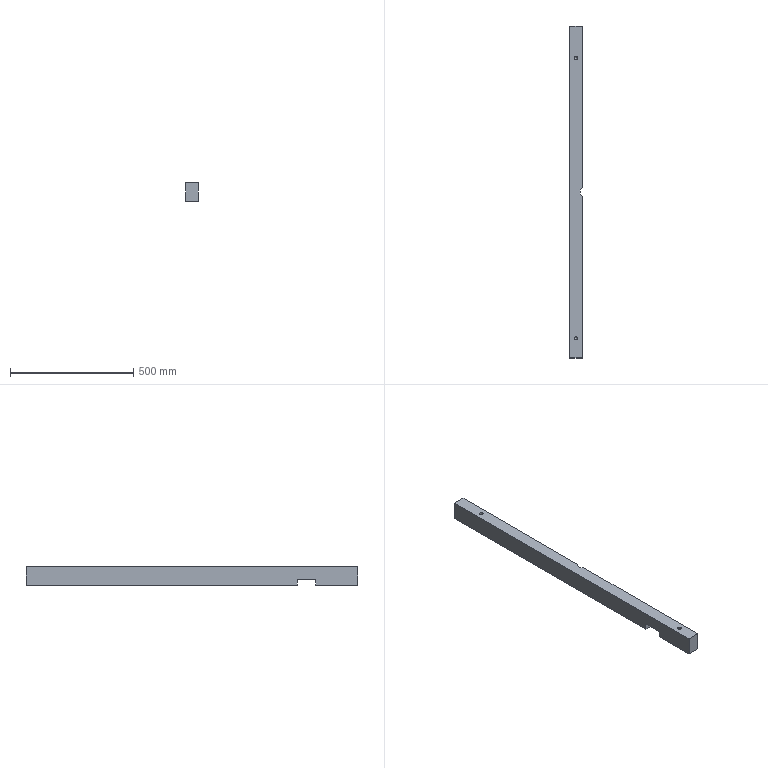Part | NX | features 3 2 | 1 solid | 20 faces | box 50 x 1345 x 75.5 mm | volume 4962481 mm3 | plane 11 | cylinder 5 | cone 4 | commonest cylinder face diameters 14.1 x4 53 x1
STEP:
#1=CARTESIAN_POINT('',(2167.05,542.5,256.5));
#2=VERTEX_POINT('',#1);
#3=CARTESIAN_POINT('',(2160.,542.5,256.5));
#4=DIRECTION('',(0.,0.,-1.));
#5=DIRECTION('',(1.,0.,0.));
#6=AXIS2_PLACEMENT_3D('',#3,#4,#5);
#7=CIRCLE('',#6,7.05);
#8=EDGE_CURVE('',#2,#2,#7,.T.);
#9=ORIENTED_EDGE('',*,*,#8,.T.);
#10=EDGE_LOOP('',(#9));
#11=FACE_BOUND('',#10,.T.);
#12=CARTESIAN_POINT('',(2185.,19.449,256.5));
#13=VERTEX_POINT('',#12);
#14=CARTESIAN_POINT('',(2185.,-19.449,256.5));
#15=VERTEX_POINT('',#14);
#16=CARTESIAN_POINT('',(2203.,0.,256.5));
#17=DIRECTION('',(0.,0.,1.));
#18=DIRECTION('',(1.,0.,0.));
#19=AXIS2_PLACEMENT_3D('',#16,#17,#18);
#20=CIRCLE('',#19,26.5);
#21=EDGE_CURVE('',#13,#15,#20,.T.);
#22=ORIENTED_EDGE('',*,*,#21,.F.);
#23=CARTESIAN_POINT('',(2185.,672.5,256.5));
#24=VERTEX_POINT('',#23);
#25=CARTESIAN_POINT('',(2185.,193.,256.5));
#26=DIRECTION('',(0.,1.,0.));
#27=VECTOR('',#26,1000.);
#28=LINE('',#25,#27);
#29=EDGE_CURVE('',#13,#24,#28,.T.);
#30=ORIENTED_EDGE('',*,*,#29,.T.);
#31=CARTESIAN_POINT('',(2135.,672.5,256.5));
#32=VERTEX_POINT('',#31);
#33=CARTESIAN_POINT('',(145.,672.5,256.5));
#34=DIRECTION('',(-1.,0.,0.));
#35=VECTOR('',#34,1000.);
#36=LINE('',#33,#35);
#37=EDGE_CURVE('',#24,#32,#36,.T.);
#38=ORIENTED_EDGE('',*,*,#37,.T.);
#39=CARTESIAN_POINT('',(2135.,-672.5,256.5));
#40=VERTEX_POINT('',#39);
#41=CARTESIAN_POINT('',(2135.,193.,256.5));
#42=DIRECTION('',(0.,-1.,0.));
#43=VECTOR('',#42,1000.);
#44=LINE('',#41,#43);
#45=EDGE_CURVE('',#32,#40,#44,.T.);
#46=ORIENTED_EDGE('',*,*,#45,.T.);
#47=CARTESIAN_POINT('',(2185.,-672.5,256.5));
#48=VERTEX_POINT('',#47);
#49=CARTESIAN_POINT('',(145.,-672.5,256.5));
#50=DIRECTION('',(1.,0.,0.));
#51=VECTOR('',#50,1000.);
#52=LINE('',#49,#51);
#53=EDGE_CURVE('',#40,#48,#52,.T.);
#54=ORIENTED_EDGE('',*,*,#53,.T.);
#55=CARTESIAN_POINT('',(2185.,193.,256.5));
#56=DIRECTION('',(0.,1.,0.));
#57=VECTOR('',#56,1000.);
#58=LINE('',#55,#57);
#59=EDGE_CURVE('',#48,#15,#58,.T.);
#60=ORIENTED_EDGE('',*,*,#59,.T.);
#61=EDGE_LOOP('',(#22,#30,#38,#46,#54,#60));
#62=FACE_BOUND('',#61,.T.);
#63=CARTESIAN_POINT('',(2167.05,-592.5,256.5));
#64=VERTEX_POINT('',#63);
#65=CARTESIAN_POINT('',(2160.,-592.5,256.5));
#66=DIRECTION('',(0.,0.,-1.));
#67=DIRECTION('',(1.,0.,0.));
#68=AXIS2_PLACEMENT_3D('',#65,#66,#67);
#69=CIRCLE('',#68,7.05);
#70=EDGE_CURVE('',#64,#64,#69,.T.);
#71=ORIENTED_EDGE('',*,*,#70,.T.);
#72=EDGE_LOOP('',(#71));
#73=FACE_BOUND('',#72,.T.);
#74=CARTESIAN_POINT('',(145.,0.,256.5));
#75=DIRECTION('',(0.,0.,1.));
#76=DIRECTION('',(1.,0.,0.));
#77=AXIS2_PLACEMENT_3D('',#74,#75,#76);
#78=PLANE('',#77);
#79=ADVANCED_FACE('',(#11,#62,#73),#78,.T.);
#80=CARTESIAN_POINT('',(2185.,-502.,181.));
#81=VERTEX_POINT('',#80);
#82=CARTESIAN_POINT('',(2135.,-502.,181.));
#83=VERTEX_POINT('',#82);
#84=CARTESIAN_POINT('',(915.,-502.,181.));
#85=DIRECTION('',(-1.,0.,0.));
#86=VECTOR('',#85,1000.);
#87=LINE('',#84,#86);
#88=EDGE_CURVE('',#81,#83,#87,.T.);
#89=ORIENTED_EDGE('',*,*,#88,.F.);
#90=CARTESIAN_POINT('',(2185.,-672.5,181.));
#91=VERTEX_POINT('',#90);
#92=CARTESIAN_POINT('',(2185.,193.,181.));
#93=DIRECTION('',(0.,-1.,0.));
#94=VECTOR('',#93,1000.);
#95=LINE('',#92,#94);
#96=EDGE_CURVE('',#81,#91,#95,.T.);
#97=ORIENTED_EDGE('',*,*,#96,.T.);
#98=CARTESIAN_POINT('',(2135.,-672.5,181.));
#99=VERTEX_POINT('',#98);
#100=CARTESIAN_POINT('',(282.5,-672.5,181.));
#101=DIRECTION('',(1.,0.,0.));
#102=VECTOR('',#101,1000.);
#103=LINE('',#100,#102);
#104=EDGE_CURVE('',#99,#91,#103,.T.);
#105=ORIENTED_EDGE('',*,*,#104,.F.);
#106=CARTESIAN_POINT('',(2135.,193.,181.));
#107=DIRECTION('',(0.,1.,0.));
#108=VECTOR('',#107,1000.);
#109=LINE('',#106,#108);
#110=EDGE_CURVE('',#99,#83,#109,.T.);
#111=ORIENTED_EDGE('',*,*,#110,.T.);
#112=EDGE_LOOP('',(#89,#97,#105,#111));
#113=FACE_BOUND('',#112,.T.);
#114=CARTESIAN_POINT('',(2167.05,-592.5,181.));
#115=VERTEX_POINT('',#114);
#116=CARTESIAN_POINT('',(2160.,-592.5,181.));
#117=DIRECTION('',(0.,0.,1.));
#118=DIRECTION('',(1.,0.,0.));
#119=AXIS2_PLACEMENT_3D('',#116,#117,#118);
#120=CIRCLE('',#119,7.05);
#121=EDGE_CURVE('',#115,#115,#120,.T.);
#122=ORIENTED_EDGE('',*,*,#121,.T.);
#123=EDGE_LOOP('',(#122));
#124=FACE_BOUND('',#123,.T.);
#125=CARTESIAN_POINT('',(915.,193.,181.));
#126=DIRECTION('',(0.,0.,-1.));
#127=DIRECTION('',(1.,0.,0.));
#128=AXIS2_PLACEMENT_3D('',#125,#126,#127);
#129=PLANE('',#128);
#130=ADVANCED_FACE('',(#113,#124),#129,.T.);
#131=CARTESIAN_POINT('',(2185.,-19.449,181.));
#132=VERTEX_POINT('',#131);
#133=CARTESIAN_POINT('',(2185.,19.449,181.));
#134=VERTEX_POINT('',#133);
#135=CARTESIAN_POINT('',(2203.,0.,181.));
#136=DIRECTION('',(0.,0.,-1.));
#137=DIRECTION('',(-1.,0.,0.));
#138=AXIS2_PLACEMENT_3D('',#135,#136,#137);
#139=CIRCLE('',#138,26.5);
#140=EDGE_CURVE('',#132,#134,#139,.T.);
#141=ORIENTED_EDGE('',*,*,#140,.F.);
#142=CARTESIAN_POINT('',(2185.,-426.,181.));
#143=VERTEX_POINT('',#142);
#144=CARTESIAN_POINT('',(2185.,193.,181.));
#145=DIRECTION('',(0.,-1.,0.));
#146=VECTOR('',#145,1000.);
#147=LINE('',#144,#146);
#148=EDGE_CURVE('',#132,#143,#147,.T.);
#149=ORIENTED_EDGE('',*,*,#148,.T.);
#150=CARTESIAN_POINT('',(2135.,-426.,181.));
#151=VERTEX_POINT('',#150);
#152=CARTESIAN_POINT('',(915.,-426.,181.));
#153=DIRECTION('',(1.,0.,0.));
#154=VECTOR('',#153,1000.);
#155=LINE('',#152,#154);
#156=EDGE_CURVE('',#151,#143,#155,.T.);
#157=ORIENTED_EDGE('',*,*,#156,.F.);
#158=CARTESIAN_POINT('',(2135.,672.5,181.));
#159=VERTEX_POINT('',#158);
#160=CARTESIAN_POINT('',(2135.,193.,181.));
#161=DIRECTION('',(0.,1.,0.));
#162=VECTOR('',#161,1000.);
#163=LINE('',#160,#162);
#164=EDGE_CURVE('',#151,#159,#163,.T.);
#165=ORIENTED_EDGE('',*,*,#164,.T.);
#166=CARTESIAN_POINT('',(2185.,672.5,181.));
#167=VERTEX_POINT('',#166);
#168=CARTESIAN_POINT('',(2185.,672.5,181.));
#169=DIRECTION('',(-1.,0.,0.));
#170=VECTOR('',#169,1000.);
#171=LINE('',#168,#170);
#172=EDGE_CURVE('',#167,#159,#171,.T.);
#173=ORIENTED_EDGE('',*,*,#172,.F.);
#174=CARTESIAN_POINT('',(2185.,193.,181.));
#175=DIRECTION('',(0.,-1.,0.));
#176=VECTOR('',#175,1000.);
#177=LINE('',#174,#176);
#178=EDGE_CURVE('',#167,#134,#177,.T.);
#179=ORIENTED_EDGE('',*,*,#178,.T.);
#180=EDGE_LOOP('',(#141,#149,#157,#165,#173,#179));
#181=FACE_BOUND('',#180,.T.);
#182=CARTESIAN_POINT('',(2167.05,542.5,181.));
#183=VERTEX_POINT('',#182);
#184=CARTESIAN_POINT('',(2160.,542.5,181.));
#185=DIRECTION('',(0.,0.,1.));
#186=DIRECTION('',(1.,0.,0.));
#187=AXIS2_PLACEMENT_3D('',#184,#185,#186);
#188=CIRCLE('',#187,7.05);
#189=EDGE_CURVE('',#183,#183,#188,.T.);
#190=ORIENTED_EDGE('',*,*,#189,.T.);
#191=EDGE_LOOP('',(#190));
#192=FACE_BOUND('',#191,.T.);
#193=CARTESIAN_POINT('',(915.,193.,181.));
#194=DIRECTION('',(0.,0.,-1.));
#195=DIRECTION('',(1.,0.,0.));
#196=AXIS2_PLACEMENT_3D('',#193,#194,#195);
#197=PLANE('',#196);
#198=ADVANCED_FACE('',(#181,#192),#197,.T.);
#199=CARTESIAN_POINT('',(2185.,19.449,-181.));
#200=DIRECTION('',(0.,0.,1.));
#201=VECTOR('',#200,1000.);
#202=LINE('',#199,#201);
#203=EDGE_CURVE('',#134,#13,#202,.T.);
#204=ORIENTED_EDGE('',*,*,#203,.F.);
#205=ORIENTED_EDGE('',*,*,#178,.F.);
#206=CARTESIAN_POINT('',(2185.,672.5,231.5));
#207=DIRECTION('',(0.,0.,-1.));
#208=VECTOR('',#207,1000.);
#209=LINE('',#206,#208);
#210=EDGE_CURVE('',#24,#167,#209,.T.);
#211=ORIENTED_EDGE('',*,*,#210,.F.);
#212=ORIENTED_EDGE('',*,*,#29,.F.);
#213=EDGE_LOOP('',(#204,#205,#211,#212));
#214=FACE_BOUND('',#213,.T.);
#215=CARTESIAN_POINT('',(2185.,193.,-1.5));
#216=DIRECTION('',(1.,0.,0.));
#217=DIRECTION('',(0.,0.,-1.));
#218=AXIS2_PLACEMENT_3D('',#215,#216,#217);
#219=PLANE('',#218);
#220=ADVANCED_FACE('',(#214),#219,.T.);
#221=CARTESIAN_POINT('',(2185.,-19.449,256.5));
#222=DIRECTION('',(0.,0.,-1.));
#223=VECTOR('',#222,1000.);
#224=LINE('',#221,#223);
#225=EDGE_CURVE('',#15,#132,#224,.T.);
#226=ORIENTED_EDGE('',*,*,#225,.F.);
#227=ORIENTED_EDGE('',*,*,#59,.F.);
#228=CARTESIAN_POINT('',(2185.,-672.5,-103.));
#229=DIRECTION('',(0.,0.,1.));
#230=VECTOR('',#229,1000.);
#231=LINE('',#228,#230);
#232=EDGE_CURVE('',#91,#48,#231,.T.);
#233=ORIENTED_EDGE('',*,*,#232,.F.);
#234=ORIENTED_EDGE('',*,*,#96,.F.);
#235=CARTESIAN_POINT('',(2185.,-502.,205.));
#236=VERTEX_POINT('',#235);
#237=CARTESIAN_POINT('',(2185.,-502.,-1.5));
#238=DIRECTION('',(0.,0.,-1.));
#239=VECTOR('',#238,1000.);
#240=LINE('',#237,#239);
#241=EDGE_CURVE('',#236,#81,#240,.T.);
#242=ORIENTED_EDGE('',*,*,#241,.F.);
#243=CARTESIAN_POINT('',(2185.,-426.,205.));
#244=VERTEX_POINT('',#243);
#245=CARTESIAN_POINT('',(2185.,193.,205.));
#246=DIRECTION('',(0.,-1.,0.));
#247=VECTOR('',#246,1000.);
#248=LINE('',#245,#247);
#249=EDGE_CURVE('',#244,#236,#248,.T.);
#250=ORIENTED_EDGE('',*,*,#249,.F.);
#251=CARTESIAN_POINT('',(2185.,-426.,-1.5));
#252=DIRECTION('',(0.,0.,1.));
#253=VECTOR('',#252,1000.);
#254=LINE('',#251,#253);
#255=EDGE_CURVE('',#143,#244,#254,.T.);
#256=ORIENTED_EDGE('',*,*,#255,.F.);
#257=ORIENTED_EDGE('',*,*,#148,.F.);
#258=EDGE_LOOP('',(#226,#227,#233,#234,#242,#250,#256,#257));
#259=FACE_BOUND('',#258,.T.);
#260=CARTESIAN_POINT('',(2185.,193.,-1.5));
#261=DIRECTION('',(1.,0.,0.));
#262=DIRECTION('',(0.,0.,-1.));
#263=AXIS2_PLACEMENT_3D('',#260,#261,#262);
#264=PLANE('',#263);
#265=ADVANCED_FACE('',(#259),#264,.T.);
#266=CARTESIAN_POINT('',(2135.,-502.,205.));
#267=VERTEX_POINT('',#266);
#268=CARTESIAN_POINT('',(2135.,-502.,-1.5));
#269=DIRECTION('',(0.,0.,1.));
#270=VECTOR('',#269,1000.);
#271=LINE('',#268,#270);
#272=EDGE_CURVE('',#83,#267,#271,.T.);
#273=ORIENTED_EDGE('',*,*,#272,.F.);
#274=ORIENTED_EDGE('',*,*,#110,.F.);
#275=CARTESIAN_POINT('',(2135.,-672.5,-103.));
#276=DIRECTION('',(0.,0.,-1.));
#277=VECTOR('',#276,1000.);
#278=LINE('',#275,#277);
#279=EDGE_CURVE('',#40,#99,#278,.T.);
#280=ORIENTED_EDGE('',*,*,#279,.F.);
#281=ORIENTED_EDGE('',*,*,#45,.F.);
#282=CARTESIAN_POINT('',(2135.,672.5,231.5));
#283=DIRECTION('',(0.,0.,1.));
#284=VECTOR('',#283,1000.);
#285=LINE('',#282,#284);
#286=EDGE_CURVE('',#159,#32,#285,.T.);
#287=ORIENTED_EDGE('',*,*,#286,.F.);
#288=ORIENTED_EDGE('',*,*,#164,.F.);
#289=CARTESIAN_POINT('',(2135.,-426.,205.));
#290=VERTEX_POINT('',#289);
#291=CARTESIAN_POINT('',(2135.,-426.,-1.5));
#292=DIRECTION('',(0.,0.,-1.));
#293=VECTOR('',#292,1000.);
#294=LINE('',#291,#293);
#295=EDGE_CURVE('',#290,#151,#294,.T.);
#296=ORIENTED_EDGE('',*,*,#295,.F.);
#297=CARTESIAN_POINT('',(2135.,193.,205.));
#298=DIRECTION('',(0.,1.,0.));
#299=VECTOR('',#298,1000.);
#300=LINE('',#297,#299);
#301=EDGE_CURVE('',#267,#290,#300,.T.);
#302=ORIENTED_EDGE('',*,*,#301,.F.);
#303=EDGE_LOOP('',(#273,#274,#280,#281,#287,#288,#296,#302));
#304=FACE_BOUND('',#303,.T.);
#305=CARTESIAN_POINT('',(2135.,193.,-1.5));
#306=DIRECTION('',(-1.,0.,0.));
#307=DIRECTION('',(0.,0.,1.));
#308=AXIS2_PLACEMENT_3D('',#305,#306,#307);
#309=PLANE('',#308);
#310=ADVANCED_FACE('',(#304),#309,.T.);
#311=ORIENTED_EDGE('',*,*,#279,.T.);
#312=ORIENTED_EDGE('',*,*,#104,.T.);
#313=ORIENTED_EDGE('',*,*,#232,.T.);
#314=ORIENTED_EDGE('',*,*,#53,.F.);
#315=EDGE_LOOP('',(#311,#312,#313,#314));
#316=FACE_BOUND('',#315,.T.);
#317=CARTESIAN_POINT('',(282.5,-672.5,-103.));
#318=DIRECTION('',(0.,1.,0.));
#319=DIRECTION('',(1.,0.,0.));
#320=AXIS2_PLACEMENT_3D('',#317,#318,#319);
#321=PLANE('',#320);
#322=ADVANCED_FACE('',(#316),#321,.F.);
#323=ORIENTED_EDGE('',*,*,#210,.T.);
#324=ORIENTED_EDGE('',*,*,#172,.T.);
#325=ORIENTED_EDGE('',*,*,#286,.T.);
#326=ORIENTED_EDGE('',*,*,#37,.F.);
#327=EDGE_LOOP('',(#323,#324,#325,#326));
#328=FACE_BOUND('',#327,.T.);
#329=CARTESIAN_POINT('',(2185.,672.5,231.5));
#330=DIRECTION('',(0.,1.,0.));
#331=DIRECTION('',(0.,0.,-1.));
#332=AXIS2_PLACEMENT_3D('',#329,#330,#331);
#333=PLANE('',#332);
#334=ADVANCED_FACE('',(#328),#333,.T.);
#335=ORIENTED_EDGE('',*,*,#249,.T.);
#336=CARTESIAN_POINT('',(2165.,-502.,205.));
#337=DIRECTION('',(1.,0.,0.));
#338=VECTOR('',#337,1000.);
#339=LINE('',#336,#338);
#340=EDGE_CURVE('',#267,#236,#339,.T.);
#341=ORIENTED_EDGE('',*,*,#340,.F.);
#342=ORIENTED_EDGE('',*,*,#301,.T.);
#343=CARTESIAN_POINT('',(2165.,-426.,205.));
#344=DIRECTION('',(-1.,0.,0.));
#345=VECTOR('',#344,1000.);
#346=LINE('',#343,#345);
#347=EDGE_CURVE('',#244,#290,#346,.T.);
#348=ORIENTED_EDGE('',*,*,#347,.F.);
#349=EDGE_LOOP('',(#335,#341,#342,#348));
#350=FACE_BOUND('',#349,.T.);
#351=CARTESIAN_POINT('',(2165.,-464.,205.));
#352=DIRECTION('',(0.,0.,1.));
#353=DIRECTION('',(-1.,0.,0.));
#354=AXIS2_PLACEMENT_3D('',#351,#352,#353);
#355=PLANE('',#354);
#356=ADVANCED_FACE('',(#350),#355,.F.);
#357=ORIENTED_EDGE('',*,*,#241,.T.);
#358=ORIENTED_EDGE('',*,*,#88,.T.);
#359=ORIENTED_EDGE('',*,*,#272,.T.);
#360=ORIENTED_EDGE('',*,*,#340,.T.);
#361=EDGE_LOOP('',(#357,#358,#359,#360));
#362=FACE_BOUND('',#361,.T.);
#363=CARTESIAN_POINT('',(2165.,-502.,25.));
#364=DIRECTION('',(0.,-1.,0.));
#365=DIRECTION('',(0.,0.,1.));
#366=AXIS2_PLACEMENT_3D('',#363,#364,#365);
#367=PLANE('',#366);
#368=ADVANCED_FACE('',(#362),#367,.F.);
#369=ORIENTED_EDGE('',*,*,#255,.T.);
#370=ORIENTED_EDGE('',*,*,#347,.T.);
#371=ORIENTED_EDGE('',*,*,#295,.T.);
#372=ORIENTED_EDGE('',*,*,#156,.T.);
#373=EDGE_LOOP('',(#369,#370,#371,#372));
#374=FACE_BOUND('',#373,.T.);
#375=CARTESIAN_POINT('',(2165.,-426.,25.));
#376=DIRECTION('',(0.,1.,0.));
#377=DIRECTION('',(0.,0.,-1.));
#378=AXIS2_PLACEMENT_3D('',#375,#376,#377);
#379=PLANE('',#378);
#380=ADVANCED_FACE('',(#374),#379,.F.);
#381=ORIENTED_EDGE('',*,*,#21,.T.);
#382=ORIENTED_EDGE('',*,*,#225,.T.);
#383=ORIENTED_EDGE('',*,*,#140,.T.);
#384=ORIENTED_EDGE('',*,*,#203,.T.);
#385=EDGE_LOOP('',(#381,#382,#383,#384));
#386=FACE_BOUND('',#385,.T.);
#387=CARTESIAN_POINT('',(2203.,0.,-181.));
#388=DIRECTION('',(0.,0.,1.));
#389=DIRECTION('',(-1.,0.,0.));
#390=AXIS2_PLACEMENT_3D('',#387,#388,#389);
#391=CYLINDRICAL_SURFACE('',#390,26.5);
#392=ADVANCED_FACE('',(#386),#391,.F.);
#393=CARTESIAN_POINT('',(2167.05,542.5,188.95));
#394=VERTEX_POINT('',#393);
#395=CARTESIAN_POINT('',(2160.,542.5,188.95));
#396=DIRECTION('',(0.,0.,1.));
#397=DIRECTION('',(1.,0.,0.));
#398=AXIS2_PLACEMENT_3D('',#395,#396,#397);
#399=CIRCLE('',#398,7.05);
#400=EDGE_CURVE('',#394,#394,#399,.T.);
#401=ORIENTED_EDGE('',*,*,#400,.T.);
#402=EDGE_LOOP('',(#401));
#403=FACE_BOUND('',#402,.T.);
#404=ORIENTED_EDGE('',*,*,#189,.F.);
#405=EDGE_LOOP('',(#404));
#406=FACE_BOUND('',#405,.T.);
#407=CARTESIAN_POINT('',(2160.,542.5,181.));
#408=DIRECTION('',(0.,0.,1.));
#409=DIRECTION('',(-1.,0.,0.));
#410=AXIS2_PLACEMENT_3D('',#407,#408,#409);
#411=CYLINDRICAL_SURFACE('',#410,7.05);
#412=ADVANCED_FACE('',(#403,#406),#411,.F.);
#413=CARTESIAN_POINT('',(2160.,542.5,196.));
#414=VERTEX_POINT('',#413);
#415=VERTEX_LOOP('',#414);
#416=FACE_BOUND('',#415,.T.);
#417=ORIENTED_EDGE('',*,*,#400,.F.);
#418=EDGE_LOOP('',(#417));
#419=FACE_BOUND('',#418,.T.);
#420=CARTESIAN_POINT('',(2160.,542.5,188.95));
#421=DIRECTION('',(0.,0.,-1.));
#422=DIRECTION('',(1.,0.,0.));
#423=AXIS2_PLACEMENT_3D('',#420,#421,#422);
#424=CONICAL_SURFACE('',#423,7.05,0.7854);
#425=ADVANCED_FACE('',(#416,#419),#424,.F.);
#426=CARTESIAN_POINT('',(2167.05,-592.5,188.95));
#427=VERTEX_POINT('',#426);
#428=CARTESIAN_POINT('',(2160.,-592.5,188.95));
#429=DIRECTION('',(0.,0.,1.));
#430=DIRECTION('',(1.,0.,0.));
#431=AXIS2_PLACEMENT_3D('',#428,#429,#430);
#432=CIRCLE('',#431,7.05);
#433=EDGE_CURVE('',#427,#427,#432,.T.);
#434=ORIENTED_EDGE('',*,*,#433,.T.);
#435=EDGE_LOOP('',(#434));
#436=FACE_BOUND('',#435,.T.);
#437=ORIENTED_EDGE('',*,*,#121,.F.);
#438=EDGE_LOOP('',(#437));
#439=FACE_BOUND('',#438,.T.);
#440=CARTESIAN_POINT('',(2160.,-592.5,181.));
#441=DIRECTION('',(0.,0.,1.));
#442=DIRECTION('',(-1.,0.,0.));
#443=AXIS2_PLACEMENT_3D('',#440,#441,#442);
#444=CYLINDRICAL_SURFACE('',#443,7.05);
#445=ADVANCED_FACE('',(#436,#439),#444,.F.);
#446=CARTESIAN_POINT('',(2160.,-592.5,196.));
#447=VERTEX_POINT('',#446);
#448=VERTEX_LOOP('',#447);
#449=FACE_BOUND('',#448,.T.);
#450=ORIENTED_EDGE('',*,*,#433,.F.);
#451=EDGE_LOOP('',(#450));
#452=FACE_BOUND('',#451,.T.);
#453=CARTESIAN_POINT('',(2160.,-592.5,188.95));
#454=DIRECTION('',(0.,0.,-1.));
#455=DIRECTION('',(1.,0.,0.));
#456=AXIS2_PLACEMENT_3D('',#453,#454,#455);
#457=CONICAL_SURFACE('',#456,7.05,0.7854);
#458=ADVANCED_FACE('',(#449,#452),#457,.F.);
#459=CARTESIAN_POINT('',(2152.95,542.5,248.55));
#460=VERTEX_POINT('',#459);
#461=CARTESIAN_POINT('',(2160.,542.5,248.55));
#462=DIRECTION('',(0.,0.,-1.));
#463=DIRECTION('',(-1.,0.,0.));
#464=AXIS2_PLACEMENT_3D('',#461,#462,#463);
#465=CIRCLE('',#464,7.05);
#466=EDGE_CURVE('',#460,#460,#465,.T.);
#467=ORIENTED_EDGE('',*,*,#466,.T.);
#468=EDGE_LOOP('',(#467));
#469=FACE_BOUND('',#468,.T.);
#470=ORIENTED_EDGE('',*,*,#8,.F.);
#471=EDGE_LOOP('',(#470));
#472=FACE_BOUND('',#471,.T.);
#473=CARTESIAN_POINT('',(2160.,542.5,256.5));
#474=DIRECTION('',(0.,0.,-1.));
#475=DIRECTION('',(-1.,0.,0.));
#476=AXIS2_PLACEMENT_3D('',#473,#474,#475);
#477=CYLINDRICAL_SURFACE('',#476,7.05);
#478=ADVANCED_FACE('',(#469,#472),#477,.F.);
#479=CARTESIAN_POINT('',(2160.,542.5,241.5));
#480=VERTEX_POINT('',#479);
#481=VERTEX_LOOP('',#480);
#482=FACE_BOUND('',#481,.T.);
#483=ORIENTED_EDGE('',*,*,#466,.F.);
#484=EDGE_LOOP('',(#483));
#485=FACE_BOUND('',#484,.T.);
#486=CARTESIAN_POINT('',(2160.,542.5,248.55));
#487=DIRECTION('',(0.,0.,1.));
#488=DIRECTION('',(-1.,0.,0.));
#489=AXIS2_PLACEMENT_3D('',#486,#487,#488);
#490=CONICAL_SURFACE('',#489,7.05,0.7854);
#491=ADVANCED_FACE('',(#482,#485),#490,.F.);
#492=CARTESIAN_POINT('',(2152.95,-592.5,248.55));
#493=VERTEX_POINT('',#492);
#494=CARTESIAN_POINT('',(2160.,-592.5,248.55));
#495=DIRECTION('',(0.,0.,-1.));
#496=DIRECTION('',(-1.,0.,0.));
#497=AXIS2_PLACEMENT_3D('',#494,#495,#496);
#498=CIRCLE('',#497,7.05);
#499=EDGE_CURVE('',#493,#493,#498,.T.);
#500=ORIENTED_EDGE('',*,*,#499,.T.);
#501=EDGE_LOOP('',(#500));
#502=FACE_BOUND('',#501,.T.);
#503=ORIENTED_EDGE('',*,*,#70,.F.);
#504=EDGE_LOOP('',(#503));
#505=FACE_BOUND('',#504,.T.);
#506=CARTESIAN_POINT('',(2160.,-592.5,256.5));
#507=DIRECTION('',(0.,0.,-1.));
#508=DIRECTION('',(-1.,0.,0.));
#509=AXIS2_PLACEMENT_3D('',#506,#507,#508);
#510=CYLINDRICAL_SURFACE('',#509,7.05);
#511=ADVANCED_FACE('',(#502,#505),#510,.F.);
#512=CARTESIAN_POINT('',(2160.,-592.5,241.5));
#513=VERTEX_POINT('',#512);
#514=VERTEX_LOOP('',#513);
#515=FACE_BOUND('',#514,.T.);
#516=ORIENTED_EDGE('',*,*,#499,.F.);
#517=EDGE_LOOP('',(#516));
#518=FACE_BOUND('',#517,.T.);
#519=CARTESIAN_POINT('',(2160.,-592.5,248.55));
#520=DIRECTION('',(0.,0.,1.));
#521=DIRECTION('',(-1.,0.,0.));
#522=AXIS2_PLACEMENT_3D('',#519,#520,#521);
#523=CONICAL_SURFACE('',#522,7.05,0.7854);
#524=ADVANCED_FACE('',(#515,#518),#523,.F.);
#525=CLOSED_SHELL('',(#79,#130,#198,#220,#265,#310,#322,#334,#356,#368,#380,#392,#412,#425,#445,#458,#478,#491,#511,#524));
#526=MANIFOLD_SOLID_BREP('',#525);
#527=(LENGTH_UNIT()NAMED_UNIT(*)SI_UNIT(.MILLI.,.METRE.));
#528=UNCERTAINTY_MEASURE_WITH_UNIT(LENGTH_MEASURE(0.00001),#527,'','');
#529=(NAMED_UNIT(*)PLANE_ANGLE_UNIT()SI_UNIT($,.RADIAN.));
#530=(NAMED_UNIT(*)SI_UNIT($,.STERADIAN.)SOLID_ANGLE_UNIT());
#531=(GEOMETRIC_REPRESENTATION_CONTEXT(3)GLOBAL_UNCERTAINTY_ASSIGNED_CONTEXT((#528))GLOBAL_UNIT_ASSIGNED_CONTEXT((#527,#529,#530))REPRESENTATION_CONTEXT('',''));
#532=ADVANCED_BREP_SHAPE_REPRESENTATION('',(#526),#531);